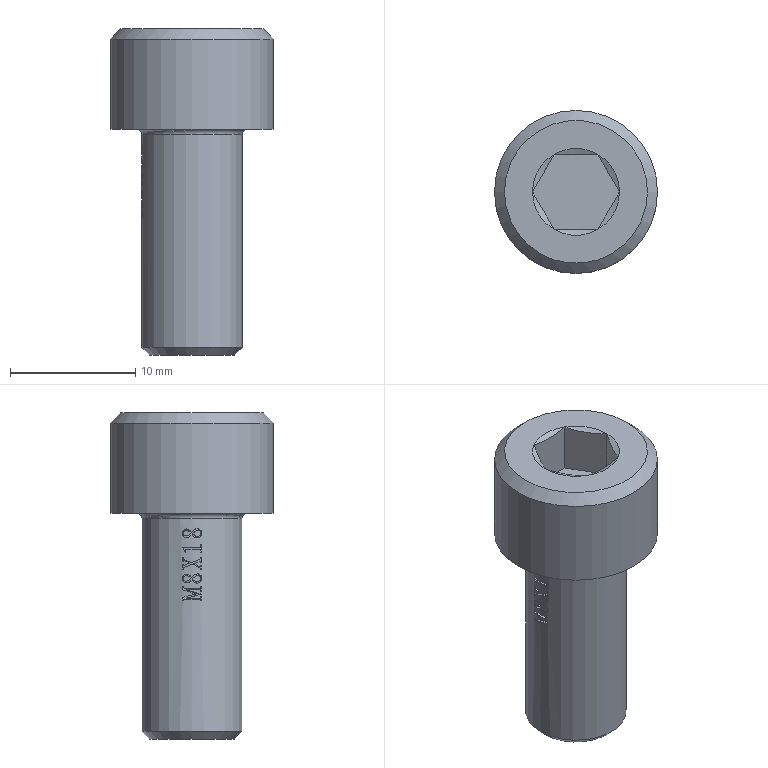Part | STEP file | solid 230 | 1 solid | 110 faces | box 13 x 13 x 26 mm | volume 1825 mm3 | plane 52 | other 40 | cylinder 9 | sphere 6 | cone 2 | torus 1 | commonest cylinder face diameters 8 x8 13 x1